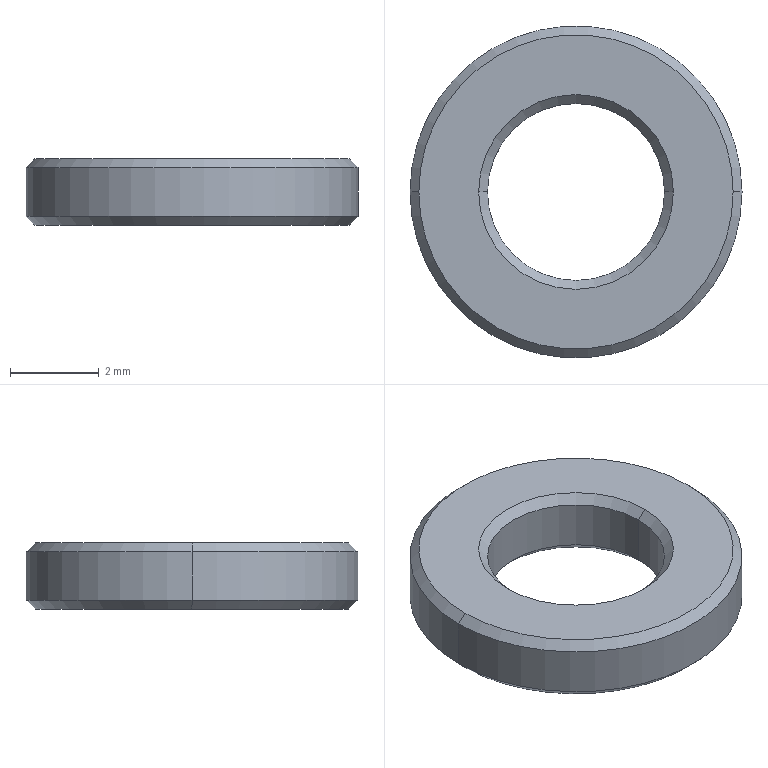Part | NX | features BREP 1 | 1 solid | 14 faces | box 7.5 x 7.5 x 1.5 mm | volume 45.973 mm3 | cone 8 | cylinder 4 | plane 2 | commonest cylinder face diameters 4 x2 7.5 x2
STEP:
#1=CARTESIAN_POINT('',(-2.2,0.,1.5));
#2=VERTEX_POINT('',#1);
#3=CARTESIAN_POINT('',(-2.,0.,1.3));
#4=VERTEX_POINT('',#3);
#5=CARTESIAN_POINT('',(-2.,0.,1.3));
#6=DIRECTION('',(-0.7071,0.,0.7071));
#7=VECTOR('',#6,1000.);
#8=LINE('',#5,#7);
#9=EDGE_CURVE('',#2,#4,#8,.F.);
#10=ORIENTED_EDGE('',*,*,#9,.T.);
#11=CARTESIAN_POINT('',(2.,0.,1.3));
#12=VERTEX_POINT('',#11);
#13=CARTESIAN_POINT('',(0.,0.,1.3));
#14=DIRECTION('',(0.,0.,1.));
#15=DIRECTION('',(1.,0.,0.));
#16=AXIS2_PLACEMENT_3D('',#13,#14,#15);
#17=CIRCLE('',#16,2.);
#18=EDGE_CURVE('',#12,#4,#17,.T.);
#19=ORIENTED_EDGE('',*,*,#18,.F.);
#20=CARTESIAN_POINT('',(2.2,0.,1.5));
#21=VERTEX_POINT('',#20);
#22=CARTESIAN_POINT('',(2.,0.,1.3));
#23=DIRECTION('',(0.7071,0.,0.7071));
#24=VECTOR('',#23,1000.);
#25=LINE('',#22,#24);
#26=EDGE_CURVE('',#21,#12,#25,.F.);
#27=ORIENTED_EDGE('',*,*,#26,.F.);
#28=CARTESIAN_POINT('',(0.,0.,1.5));
#29=DIRECTION('',(0.,0.,-1.));
#30=DIRECTION('',(1.,0.,0.));
#31=AXIS2_PLACEMENT_3D('',#28,#29,#30);
#32=CIRCLE('',#31,2.2);
#33=EDGE_CURVE('',#2,#21,#32,.T.);
#34=ORIENTED_EDGE('',*,*,#33,.F.);
#35=EDGE_LOOP('',(#10,#19,#27,#34));
#36=FACE_BOUND('',#35,.T.);
#37=CARTESIAN_POINT('',(0.,0.,1.3));
#38=DIRECTION('',(0.,0.,1.));
#39=DIRECTION('',(1.,0.,0.));
#40=AXIS2_PLACEMENT_3D('',#37,#38,#39);
#41=CONICAL_SURFACE('',#40,2.,0.7854);
#42=ADVANCED_FACE('',(#36),#41,.F.);
#43=CARTESIAN_POINT('',(3.55,0.,1.5));
#44=VERTEX_POINT('',#43);
#45=CARTESIAN_POINT('',(3.75,0.,1.3));
#46=VERTEX_POINT('',#45);
#47=CARTESIAN_POINT('',(3.55,0.,1.5));
#48=DIRECTION('',(0.7071,0.,-0.7071));
#49=VECTOR('',#48,1000.);
#50=LINE('',#47,#49);
#51=EDGE_CURVE('',#44,#46,#50,.T.);
#52=ORIENTED_EDGE('',*,*,#51,.F.);
#53=CARTESIAN_POINT('',(-3.55,0.,1.5));
#54=VERTEX_POINT('',#53);
#55=CARTESIAN_POINT('',(0.,0.,1.5));
#56=DIRECTION('',(0.,0.,1.));
#57=DIRECTION('',(1.,0.,0.));
#58=AXIS2_PLACEMENT_3D('',#55,#56,#57);
#59=CIRCLE('',#58,3.55);
#60=EDGE_CURVE('',#54,#44,#59,.T.);
#61=ORIENTED_EDGE('',*,*,#60,.F.);
#62=CARTESIAN_POINT('',(-3.75,0.,1.3));
#63=VERTEX_POINT('',#62);
#64=CARTESIAN_POINT('',(-3.55,0.,1.5));
#65=DIRECTION('',(-0.7071,0.,-0.7071));
#66=VECTOR('',#65,1000.);
#67=LINE('',#64,#66);
#68=EDGE_CURVE('',#54,#63,#67,.T.);
#69=ORIENTED_EDGE('',*,*,#68,.T.);
#70=CARTESIAN_POINT('',(0.,0.,1.3));
#71=DIRECTION('',(0.,0.,-1.));
#72=DIRECTION('',(1.,0.,0.));
#73=AXIS2_PLACEMENT_3D('',#70,#71,#72);
#74=CIRCLE('',#73,3.75);
#75=EDGE_CURVE('',#46,#63,#74,.T.);
#76=ORIENTED_EDGE('',*,*,#75,.F.);
#77=EDGE_LOOP('',(#52,#61,#69,#76));
#78=FACE_BOUND('',#77,.T.);
#79=CARTESIAN_POINT('',(0.,0.,1.5));
#80=DIRECTION('',(0.,0.,-1.));
#81=DIRECTION('',(-1.,0.,0.));
#82=AXIS2_PLACEMENT_3D('',#79,#80,#81);
#83=CONICAL_SURFACE('',#82,3.55,0.7854);
#84=ADVANCED_FACE('',(#78),#83,.T.);
#85=CARTESIAN_POINT('',(2.,0.,0.2));
#86=VERTEX_POINT('',#85);
#87=CARTESIAN_POINT('',(2.2,0.,0.));
#88=VERTEX_POINT('',#87);
#89=CARTESIAN_POINT('',(2.2,0.,0.));
#90=DIRECTION('',(0.7071,0.,-0.7071));
#91=VECTOR('',#90,1000.);
#92=LINE('',#89,#91);
#93=EDGE_CURVE('',#86,#88,#92,.T.);
#94=ORIENTED_EDGE('',*,*,#93,.F.);
#95=CARTESIAN_POINT('',(-2.,0.,0.2));
#96=VERTEX_POINT('',#95);
#97=CARTESIAN_POINT('',(0.,0.,0.2));
#98=DIRECTION('',(0.,0.,-1.));
#99=DIRECTION('',(1.,0.,0.));
#100=AXIS2_PLACEMENT_3D('',#97,#98,#99);
#101=CIRCLE('',#100,2.);
#102=EDGE_CURVE('',#96,#86,#101,.T.);
#103=ORIENTED_EDGE('',*,*,#102,.F.);
#104=CARTESIAN_POINT('',(-2.2,0.,0.));
#105=VERTEX_POINT('',#104);
#106=CARTESIAN_POINT('',(-2.2,0.,0.));
#107=DIRECTION('',(-0.7071,0.,-0.7071));
#108=VECTOR('',#107,1000.);
#109=LINE('',#106,#108);
#110=EDGE_CURVE('',#96,#105,#109,.T.);
#111=ORIENTED_EDGE('',*,*,#110,.T.);
#112=CARTESIAN_POINT('',(0.,0.,0.));
#113=DIRECTION('',(0.,0.,1.));
#114=DIRECTION('',(1.,0.,0.));
#115=AXIS2_PLACEMENT_3D('',#112,#113,#114);
#116=CIRCLE('',#115,2.2);
#117=EDGE_CURVE('',#88,#105,#116,.T.);
#118=ORIENTED_EDGE('',*,*,#117,.F.);
#119=EDGE_LOOP('',(#94,#103,#111,#118));
#120=FACE_BOUND('',#119,.T.);
#121=CARTESIAN_POINT('',(0.,0.,0.));
#122=DIRECTION('',(0.,0.,-1.));
#123=DIRECTION('',(-1.,0.,0.));
#124=AXIS2_PLACEMENT_3D('',#121,#122,#123);
#125=CONICAL_SURFACE('',#124,2.2,0.7854);
#126=ADVANCED_FACE('',(#120),#125,.F.);
#127=CARTESIAN_POINT('',(-3.75,0.,0.2));
#128=VERTEX_POINT('',#127);
#129=CARTESIAN_POINT('',(-3.55,0.,0.));
#130=VERTEX_POINT('',#129);
#131=CARTESIAN_POINT('',(-3.75,0.,0.2));
#132=DIRECTION('',(-0.7071,0.,0.7071));
#133=VECTOR('',#132,1000.);
#134=LINE('',#131,#133);
#135=EDGE_CURVE('',#128,#130,#134,.F.);
#136=ORIENTED_EDGE('',*,*,#135,.T.);
#137=CARTESIAN_POINT('',(3.55,0.,0.));
#138=VERTEX_POINT('',#137);
#139=CARTESIAN_POINT('',(0.,0.,0.));
#140=DIRECTION('',(0.,0.,-1.));
#141=DIRECTION('',(1.,0.,0.));
#142=AXIS2_PLACEMENT_3D('',#139,#140,#141);
#143=CIRCLE('',#142,3.55);
#144=EDGE_CURVE('',#138,#130,#143,.T.);
#145=ORIENTED_EDGE('',*,*,#144,.F.);
#146=CARTESIAN_POINT('',(3.75,0.,0.2));
#147=VERTEX_POINT('',#146);
#148=CARTESIAN_POINT('',(3.75,0.,0.2));
#149=DIRECTION('',(0.7071,0.,0.7071));
#150=VECTOR('',#149,1000.);
#151=LINE('',#148,#150);
#152=EDGE_CURVE('',#147,#138,#151,.F.);
#153=ORIENTED_EDGE('',*,*,#152,.F.);
#154=CARTESIAN_POINT('',(0.,0.,0.2));
#155=DIRECTION('',(0.,0.,1.));
#156=DIRECTION('',(1.,0.,0.));
#157=AXIS2_PLACEMENT_3D('',#154,#155,#156);
#158=CIRCLE('',#157,3.75);
#159=EDGE_CURVE('',#128,#147,#158,.T.);
#160=ORIENTED_EDGE('',*,*,#159,.F.);
#161=EDGE_LOOP('',(#136,#145,#153,#160));
#162=FACE_BOUND('',#161,.T.);
#163=CARTESIAN_POINT('',(0.,0.,0.2));
#164=DIRECTION('',(0.,0.,1.));
#165=DIRECTION('',(1.,0.,0.));
#166=AXIS2_PLACEMENT_3D('',#163,#164,#165);
#167=CONICAL_SURFACE('',#166,3.75,0.7854);
#168=ADVANCED_FACE('',(#162),#167,.T.);
#169=CARTESIAN_POINT('',(2.,0.,1.5));
#170=DIRECTION('',(0.,0.,-1.));
#171=VECTOR('',#170,1000.);
#172=LINE('',#169,#171);
#173=EDGE_CURVE('',#12,#86,#172,.T.);
#174=ORIENTED_EDGE('',*,*,#173,.F.);
#175=ORIENTED_EDGE('',*,*,#18,.T.);
#176=CARTESIAN_POINT('',(-2.,0.,1.5));
#177=DIRECTION('',(0.,0.,-1.));
#178=VECTOR('',#177,1000.);
#179=LINE('',#176,#178);
#180=EDGE_CURVE('',#4,#96,#179,.T.);
#181=ORIENTED_EDGE('',*,*,#180,.T.);
#182=ORIENTED_EDGE('',*,*,#102,.T.);
#183=EDGE_LOOP('',(#174,#175,#181,#182));
#184=FACE_BOUND('',#183,.T.);
#185=CARTESIAN_POINT('',(0.,0.,1.5));
#186=DIRECTION('',(0.,0.,-1.));
#187=DIRECTION('',(-1.,0.,0.));
#188=AXIS2_PLACEMENT_3D('',#185,#186,#187);
#189=CYLINDRICAL_SURFACE('',#188,2.);
#190=ADVANCED_FACE('',(#184),#189,.F.);
#191=CARTESIAN_POINT('',(3.75,0.,1.5));
#192=DIRECTION('',(0.,0.,-1.));
#193=VECTOR('',#192,1000.);
#194=LINE('',#191,#193);
#195=EDGE_CURVE('',#46,#147,#194,.T.);
#196=ORIENTED_EDGE('',*,*,#195,.F.);
#197=ORIENTED_EDGE('',*,*,#75,.T.);
#198=CARTESIAN_POINT('',(-3.75,0.,1.5));
#199=DIRECTION('',(0.,0.,-1.));
#200=VECTOR('',#199,1000.);
#201=LINE('',#198,#200);
#202=EDGE_CURVE('',#63,#128,#201,.T.);
#203=ORIENTED_EDGE('',*,*,#202,.T.);
#204=ORIENTED_EDGE('',*,*,#159,.T.);
#205=EDGE_LOOP('',(#196,#197,#203,#204));
#206=FACE_BOUND('',#205,.T.);
#207=CARTESIAN_POINT('',(0.,0.,1.5));
#208=DIRECTION('',(0.,0.,-1.));
#209=DIRECTION('',(-1.,0.,0.));
#210=AXIS2_PLACEMENT_3D('',#207,#208,#209);
#211=CYLINDRICAL_SURFACE('',#210,3.75);
#212=ADVANCED_FACE('',(#206),#211,.T.);
#213=CARTESIAN_POINT('',(0.,0.,0.));
#214=DIRECTION('',(0.,0.,1.));
#215=DIRECTION('',(1.,0.,0.));
#216=AXIS2_PLACEMENT_3D('',#213,#214,#215);
#217=CIRCLE('',#216,2.2);
#218=EDGE_CURVE('',#105,#88,#217,.T.);
#219=ORIENTED_EDGE('',*,*,#218,.T.);
#220=ORIENTED_EDGE('',*,*,#117,.T.);
#221=EDGE_LOOP('',(#219,#220));
#222=FACE_BOUND('',#221,.T.);
#223=ORIENTED_EDGE('',*,*,#144,.T.);
#224=CARTESIAN_POINT('',(0.,0.,0.));
#225=DIRECTION('',(0.,0.,-1.));
#226=DIRECTION('',(1.,0.,0.));
#227=AXIS2_PLACEMENT_3D('',#224,#225,#226);
#228=CIRCLE('',#227,3.55);
#229=EDGE_CURVE('',#130,#138,#228,.T.);
#230=ORIENTED_EDGE('',*,*,#229,.T.);
#231=EDGE_LOOP('',(#223,#230));
#232=FACE_BOUND('',#231,.T.);
#233=CARTESIAN_POINT('',(0.,0.,0.));
#234=DIRECTION('',(0.,0.,1.));
#235=DIRECTION('',(1.,0.,0.));
#236=AXIS2_PLACEMENT_3D('',#233,#234,#235);
#237=PLANE('',#236);
#238=ADVANCED_FACE('',(#222,#232),#237,.F.);
#239=CARTESIAN_POINT('',(0.,0.,1.5));
#240=DIRECTION('',(0.,0.,-1.));
#241=DIRECTION('',(1.,0.,0.));
#242=AXIS2_PLACEMENT_3D('',#239,#240,#241);
#243=CIRCLE('',#242,2.2);
#244=EDGE_CURVE('',#21,#2,#243,.T.);
#245=ORIENTED_EDGE('',*,*,#244,.T.);
#246=ORIENTED_EDGE('',*,*,#33,.T.);
#247=EDGE_LOOP('',(#245,#246));
#248=FACE_BOUND('',#247,.T.);
#249=ORIENTED_EDGE('',*,*,#60,.T.);
#250=CARTESIAN_POINT('',(0.,0.,1.5));
#251=DIRECTION('',(0.,0.,1.));
#252=DIRECTION('',(1.,0.,0.));
#253=AXIS2_PLACEMENT_3D('',#250,#251,#252);
#254=CIRCLE('',#253,3.55);
#255=EDGE_CURVE('',#44,#54,#254,.T.);
#256=ORIENTED_EDGE('',*,*,#255,.T.);
#257=EDGE_LOOP('',(#249,#256));
#258=FACE_BOUND('',#257,.T.);
#259=CARTESIAN_POINT('',(0.,0.,1.5));
#260=DIRECTION('',(0.,0.,1.));
#261=DIRECTION('',(1.,0.,0.));
#262=AXIS2_PLACEMENT_3D('',#259,#260,#261);
#263=PLANE('',#262);
#264=ADVANCED_FACE('',(#248,#258),#263,.T.);
#265=CARTESIAN_POINT('',(0.,0.,1.3));
#266=DIRECTION('',(0.,0.,-1.));
#267=DIRECTION('',(1.,0.,0.));
#268=AXIS2_PLACEMENT_3D('',#265,#266,#267);
#269=CIRCLE('',#268,3.75);
#270=EDGE_CURVE('',#63,#46,#269,.T.);
#271=ORIENTED_EDGE('',*,*,#270,.T.);
#272=ORIENTED_EDGE('',*,*,#195,.T.);
#273=CARTESIAN_POINT('',(0.,0.,0.2));
#274=DIRECTION('',(0.,0.,1.));
#275=DIRECTION('',(1.,0.,0.));
#276=AXIS2_PLACEMENT_3D('',#273,#274,#275);
#277=CIRCLE('',#276,3.75);
#278=EDGE_CURVE('',#147,#128,#277,.T.);
#279=ORIENTED_EDGE('',*,*,#278,.T.);
#280=ORIENTED_EDGE('',*,*,#202,.F.);
#281=EDGE_LOOP('',(#271,#272,#279,#280));
#282=FACE_BOUND('',#281,.T.);
#283=CARTESIAN_POINT('',(0.,0.,1.5));
#284=DIRECTION('',(0.,0.,-1.));
#285=DIRECTION('',(-1.,0.,0.));
#286=AXIS2_PLACEMENT_3D('',#283,#284,#285);
#287=CYLINDRICAL_SURFACE('',#286,3.75);
#288=ADVANCED_FACE('',(#282),#287,.T.);
#289=CARTESIAN_POINT('',(0.,0.,1.3));
#290=DIRECTION('',(0.,0.,1.));
#291=DIRECTION('',(1.,0.,0.));
#292=AXIS2_PLACEMENT_3D('',#289,#290,#291);
#293=CIRCLE('',#292,2.);
#294=EDGE_CURVE('',#4,#12,#293,.T.);
#295=ORIENTED_EDGE('',*,*,#294,.T.);
#296=ORIENTED_EDGE('',*,*,#173,.T.);
#297=CARTESIAN_POINT('',(0.,0.,0.2));
#298=DIRECTION('',(0.,0.,-1.));
#299=DIRECTION('',(1.,0.,0.));
#300=AXIS2_PLACEMENT_3D('',#297,#298,#299);
#301=CIRCLE('',#300,2.);
#302=EDGE_CURVE('',#86,#96,#301,.T.);
#303=ORIENTED_EDGE('',*,*,#302,.T.);
#304=ORIENTED_EDGE('',*,*,#180,.F.);
#305=EDGE_LOOP('',(#295,#296,#303,#304));
#306=FACE_BOUND('',#305,.T.);
#307=CARTESIAN_POINT('',(0.,0.,1.5));
#308=DIRECTION('',(0.,0.,-1.));
#309=DIRECTION('',(-1.,0.,0.));
#310=AXIS2_PLACEMENT_3D('',#307,#308,#309);
#311=CYLINDRICAL_SURFACE('',#310,2.);
#312=ADVANCED_FACE('',(#306),#311,.F.);
#313=ORIENTED_EDGE('',*,*,#229,.F.);
#314=ORIENTED_EDGE('',*,*,#135,.F.);
#315=ORIENTED_EDGE('',*,*,#278,.F.);
#316=ORIENTED_EDGE('',*,*,#152,.T.);
#317=EDGE_LOOP('',(#313,#314,#315,#316));
#318=FACE_BOUND('',#317,.T.);
#319=CARTESIAN_POINT('',(0.,0.,0.2));
#320=DIRECTION('',(0.,0.,1.));
#321=DIRECTION('',(1.,0.,0.));
#322=AXIS2_PLACEMENT_3D('',#319,#320,#321);
#323=CONICAL_SURFACE('',#322,3.75,0.7854);
#324=ADVANCED_FACE('',(#318),#323,.T.);
#325=ORIENTED_EDGE('',*,*,#302,.F.);
#326=ORIENTED_EDGE('',*,*,#93,.T.);
#327=ORIENTED_EDGE('',*,*,#218,.F.);
#328=ORIENTED_EDGE('',*,*,#110,.F.);
#329=EDGE_LOOP('',(#325,#326,#327,#328));
#330=FACE_BOUND('',#329,.T.);
#331=CARTESIAN_POINT('',(0.,0.,0.));
#332=DIRECTION('',(0.,0.,-1.));
#333=DIRECTION('',(-1.,0.,0.));
#334=AXIS2_PLACEMENT_3D('',#331,#332,#333);
#335=CONICAL_SURFACE('',#334,2.2,0.7854);
#336=ADVANCED_FACE('',(#330),#335,.F.);
#337=ORIENTED_EDGE('',*,*,#255,.F.);
#338=ORIENTED_EDGE('',*,*,#51,.T.);
#339=ORIENTED_EDGE('',*,*,#270,.F.);
#340=ORIENTED_EDGE('',*,*,#68,.F.);
#341=EDGE_LOOP('',(#337,#338,#339,#340));
#342=FACE_BOUND('',#341,.T.);
#343=CARTESIAN_POINT('',(0.,0.,1.5));
#344=DIRECTION('',(0.,0.,-1.));
#345=DIRECTION('',(-1.,0.,0.));
#346=AXIS2_PLACEMENT_3D('',#343,#344,#345);
#347=CONICAL_SURFACE('',#346,3.55,0.7854);
#348=ADVANCED_FACE('',(#342),#347,.T.);
#349=ORIENTED_EDGE('',*,*,#294,.F.);
#350=ORIENTED_EDGE('',*,*,#9,.F.);
#351=ORIENTED_EDGE('',*,*,#244,.F.);
#352=ORIENTED_EDGE('',*,*,#26,.T.);
#353=EDGE_LOOP('',(#349,#350,#351,#352));
#354=FACE_BOUND('',#353,.T.);
#355=CARTESIAN_POINT('',(0.,0.,1.3));
#356=DIRECTION('',(0.,0.,1.));
#357=DIRECTION('',(1.,0.,0.));
#358=AXIS2_PLACEMENT_3D('',#355,#356,#357);
#359=CONICAL_SURFACE('',#358,2.,0.7854);
#360=ADVANCED_FACE('',(#354),#359,.F.);
#361=CLOSED_SHELL('',(#42,#84,#126,#168,#190,#212,#238,#264,#288,#312,#324,#336,#348,#360));
#362=MANIFOLD_SOLID_BREP('',#361);
#363=(LENGTH_UNIT()NAMED_UNIT(*)SI_UNIT(.MILLI.,.METRE.));
#364=UNCERTAINTY_MEASURE_WITH_UNIT(LENGTH_MEASURE(0.00001),#363,'','');
#365=(NAMED_UNIT(*)PLANE_ANGLE_UNIT()SI_UNIT($,.RADIAN.));
#366=(NAMED_UNIT(*)SI_UNIT($,.STERADIAN.)SOLID_ANGLE_UNIT());
#367=(GEOMETRIC_REPRESENTATION_CONTEXT(3)GLOBAL_UNCERTAINTY_ASSIGNED_CONTEXT((#364))GLOBAL_UNIT_ASSIGNED_CONTEXT((#363,#365,#366))REPRESENTATION_CONTEXT('',''));
#368=ADVANCED_BREP_SHAPE_REPRESENTATION('',(#362),#367);